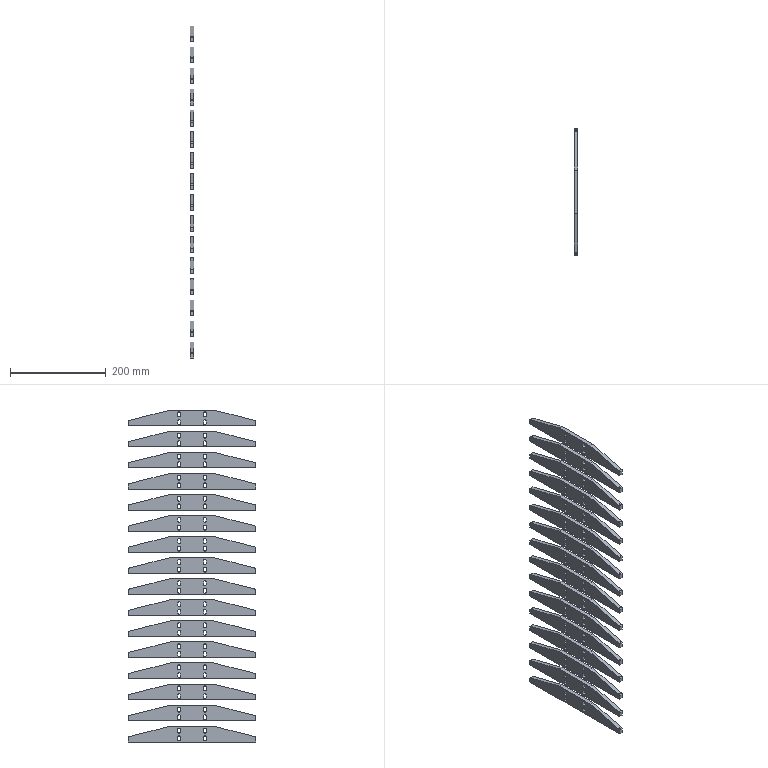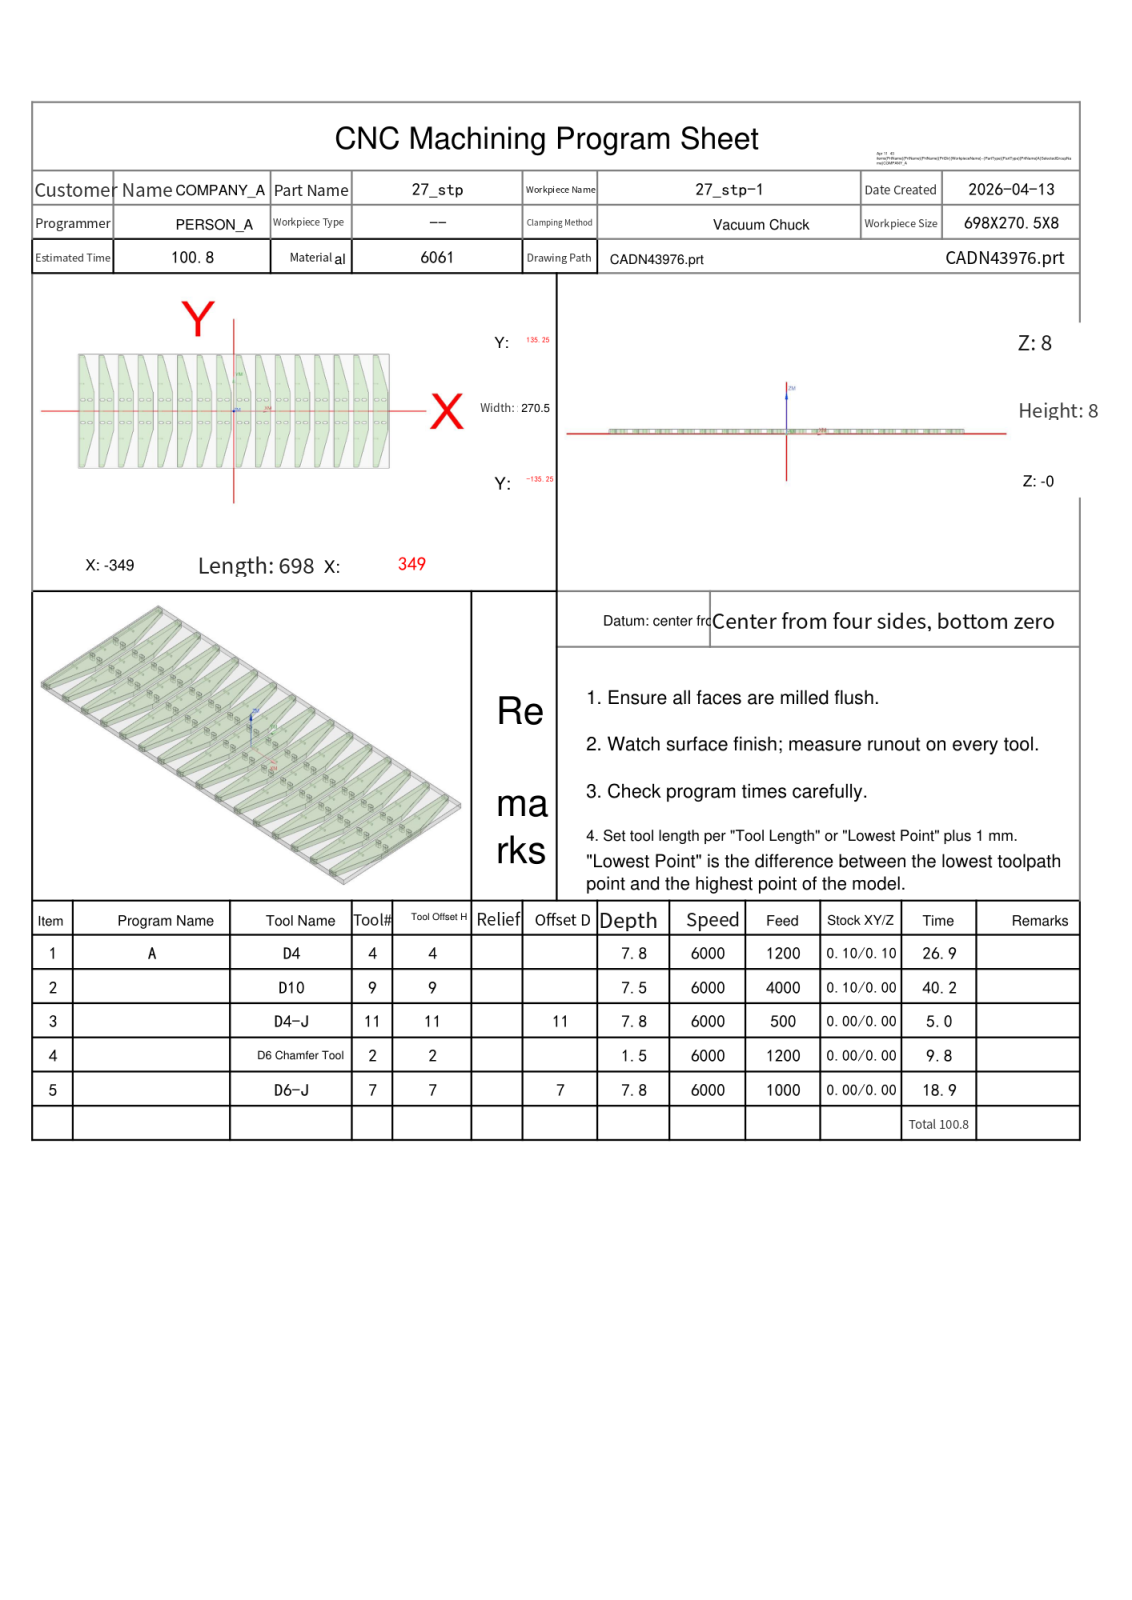NC program | NX | posted by the shop | part box 8 x 265.5 x 693 mm
Lines 17059 to 19371 of 21683, first 2178 of 2313 lines:
N3 T11 M06
(D4-J  D=4. R=0. H=11 ce=0.00 di=0.00)
G00 G90 G54 X-323. Y-27.5 M03 S6000
G43 H11 Z28.
M08
Z4.6
G01 Z4.1 F500.
G41 D11
Y-27.55
G03 X-322.8 Y-27.75 I.2 J0.0
G01 X-320.3
G03 X-319.55 Y-27. I0.0 J.75
X-320.3 Y-26.25 I-.75 J0.0
G01 X-325.3
G03 X-326.05 Y-27. I0.0 J-.75
X-325.3 Y-27.75 I.75 J0.0
G01 X-322.8
X-322.3
G03 X-322.1 Y-27.55 I0.0 J.2
G01 G40 Y-27.5
Z4.6
G00 Z9.
X-323.
Z.7
G01 Z.2
G41 D11
Y-27.55
G03 X-322.8 Y-27.75 I.2 J0.0
G01 X-320.3
G03 X-319.55 Y-27. I0.0 J.75
X-320.3 Y-26.25 I-.75 J0.0
G01 X-325.3
G03 X-326.05 Y-27. I0.0 J-.75
X-325.3 Y-27.75 I.75 J0.0
G01 X-322.8
X-322.3
G03 X-322.1 Y-27.55 I0.0 J.2
G01 G40 Y-27.5
Z.7
G00 Z28.
X-338.6 Y-26.5
Z4.6
G01 Z4.1
G41 D11
Y-26.45
G03 X-338.8 Y-26.25 I-.2 J0.0
G01 X-341.3
G03 X-342.05 Y-27. I0.0 J-.75
X-341.3 Y-27.75 I.75 J0.0
G01 X-336.3
G03 X-335.55 Y-27. I0.0 J.75
X-336.3 Y-26.25 I-.75 J0.0
G01 X-338.8
X-339.3
G03 X-339.5 Y-26.45 I0.0 J-.2
G01 G40 Y-26.5
Z4.6
G00 Z9.
X-338.6
Z.7
G01 Z.2
G41 D11
Y-26.45
G03 X-338.8 Y-26.25 I-.2 J0.0
G01 X-341.3
G03 X-342.05 Y-27. I0.0 J-.75
X-341.3 Y-27.75 I.75 J0.0
G01 X-336.3
G03 X-335.55 Y-27. I0.0 J.75
X-336.3 Y-26.25 I-.75 J0.0
G01 X-338.8
X-339.3
G03 X-339.5 Y-26.45 I0.0 J-.2
G01 G40 Y-26.5
Z.7
G00 Z28.
X-278.6
Z4.6
G01 Z4.1
G41 D11
Y-26.45
G03 X-278.8 Y-26.25 I-.2 J0.0
G01 X-281.3
G03 X-282.05 Y-27. I0.0 J-.75
X-281.3 Y-27.75 I.75 J0.0
G01 X-276.3
G03 X-275.55 Y-27. I0.0 J.75
X-276.3 Y-26.25 I-.75 J0.0
G01 X-278.8
X-279.3
G03 X-279.5 Y-26.45 I0.0 J-.2
G01 G40 Y-26.5
Z4.6
G00 Z9.
X-278.6
Z.7
G01 Z.2
G41 D11
Y-26.45
G03 X-278.8 Y-26.25 I-.2 J0.0
G01 X-281.3
G03 X-282.05 Y-27. I0.0 J-.75
X-281.3 Y-27.75 I.75 J0.0
G01 X-276.3
G03 X-275.55 Y-27. I0.0 J.75
X-276.3 Y-26.25 I-.75 J0.0
G01 X-278.8
X-279.3
G03 X-279.5 Y-26.45 I0.0 J-.2
G01 G40 Y-26.5
Z.7
G00 Z28.
X-294.6
Z4.6
G01 Z4.1
G41 D11
Y-26.45
G03 X-294.8 Y-26.25 I-.2 J0.0
G01 X-297.3
G03 X-298.05 Y-27. I0.0 J-.75
X-297.3 Y-27.75 I.75 J0.0
G01 X-292.3
G03 X-291.55 Y-27. I0.0 J.75
X-292.3 Y-26.25 I-.75 J0.0
G01 X-294.8
X-295.3
G03 X-295.5 Y-26.45 I0.0 J-.2
G01 G40 Y-26.5
Z4.6
G00 Z9.
X-294.6
Z.7
G01 Z.2
G41 D11
Y-26.45
G03 X-294.8 Y-26.25 I-.2 J0.0
G01 X-297.3
G03 X-298.05 Y-27. I0.0 J-.75
X-297.3 Y-27.75 I.75 J0.0
G01 X-292.3
G03 X-291.55 Y-27. I0.0 J.75
X-292.3 Y-26.25 I-.75 J0.0
G01 X-294.8
X-295.3
G03 X-295.5 Y-26.45 I0.0 J-.2
G01 G40 Y-26.5
Z.7
G00 Z28.
X-235. Y-27.5
Z4.6
G01 Z4.1
G41 D11
Y-27.55
G03 X-234.8 Y-27.75 I.2 J0.0
G01 X-232.3
G03 X-231.55 Y-27. I0.0 J.75
X-232.3 Y-26.25 I-.75 J0.0
G01 X-237.3
G03 X-238.05 Y-27. I0.0 J-.75
X-237.3 Y-27.75 I.75 J0.0
G01 X-234.8
X-234.3
G03 X-234.1 Y-27.55 I0.0 J.2
G01 G40 Y-27.5
Z4.6
G00 Z9.
X-235.
Z.7
G01 Z.2
G41 D11
Y-27.55
G03 X-234.8 Y-27.75 I.2 J0.0
G01 X-232.3
G03 X-231.55 Y-27. I0.0 J.75
X-232.3 Y-26.25 I-.75 J0.0
G01 X-237.3
G03 X-238.05 Y-27. I0.0 J-.75
X-237.3 Y-27.75 I.75 J0.0
G01 X-234.8
X-234.3
G03 X-234.1 Y-27.55 I0.0 J.2
G01 G40 Y-27.5
Z.7
G00 Z28.
X-251.
Z4.6
G01 Z4.1
G41 D11
Y-27.55
G03 X-250.8 Y-27.75 I.2 J0.0
G01 X-248.3
G03 X-247.55 Y-27. I0.0 J.75
X-248.3 Y-26.25 I-.75 J0.0
G01 X-253.3
G03 X-254.05 Y-27. I0.0 J-.75
X-253.3 Y-27.75 I.75 J0.0
G01 X-250.8
X-250.3
G03 X-250.1 Y-27.55 I0.0 J.2
G01 G40 Y-27.5
Z4.6
G00 Z9.
X-251.
Z.7
G01 Z.2
G41 D11
Y-27.55
G03 X-250.8 Y-27.75 I.2 J0.0
G01 X-248.3
G03 X-247.55 Y-27. I0.0 J.75
X-248.3 Y-26.25 I-.75 J0.0
G01 X-253.3
G03 X-254.05 Y-27. I0.0 J-.75
X-253.3 Y-27.75 I.75 J0.0
G01 X-250.8
X-250.3
G03 X-250.1 Y-27.55 I0.0 J.2
G01 G40 Y-27.5
Z.7
G00 Z28.
X-191.
Z4.6
G01 Z4.1
G41 D11
Y-27.55
G03 X-190.8 Y-27.75 I.2 J0.0
G01 X-188.3
G03 X-187.55 Y-27. I0.0 J.75
X-188.3 Y-26.25 I-.75 J0.0
G01 X-193.3
G03 X-194.05 Y-27. I0.0 J-.75
X-193.3 Y-27.75 I.75 J0.0
G01 X-190.8
X-190.3
G03 X-190.1 Y-27.55 I0.0 J.2
G01 G40 Y-27.5
Z4.6
G00 Z9.
X-191.
Z.7
G01 Z.2
G41 D11
Y-27.55
G03 X-190.8 Y-27.75 I.2 J0.0
G01 X-188.3
G03 X-187.55 Y-27. I0.0 J.75
X-188.3 Y-26.25 I-.75 J0.0
G01 X-193.3
G03 X-194.05 Y-27. I0.0 J-.75
X-193.3 Y-27.75 I.75 J0.0
G01 X-190.8
X-190.3
G03 X-190.1 Y-27.55 I0.0 J.2
G01 G40 Y-27.5
Z.7
G00 Z28.
X-207.
Z4.6
G01 Z4.1
G41 D11
Y-27.55
G03 X-206.8 Y-27.75 I.2 J0.0
G01 X-204.3
G03 X-203.55 Y-27. I0.0 J.75
X-204.3 Y-26.25 I-.75 J0.0
G01 X-209.3
G03 X-210.05 Y-27. I0.0 J-.75
X-209.3 Y-27.75 I.75 J0.0
G01 X-206.8
X-206.3
G03 X-206.1 Y-27.55 I0.0 J.2
G01 G40 Y-27.5
Z4.6
G00 Z9.
X-207.
Z.7
G01 Z.2
G41 D11
Y-27.55
G03 X-206.8 Y-27.75 I.2 J0.0
G01 X-204.3
G03 X-203.55 Y-27. I0.0 J.75
X-204.3 Y-26.25 I-.75 J0.0
G01 X-209.3
G03 X-210.05 Y-27. I0.0 J-.75
X-209.3 Y-27.75 I.75 J0.0
G01 X-206.8
X-206.3
G03 X-206.1 Y-27.55 I0.0 J.2
G01 G40 Y-27.5
Z.7
G00 Z28.
X-147.
Z4.6
G01 Z4.1
G41 D11
Y-27.55
G03 X-146.8 Y-27.75 I.2 J0.0
G01 X-144.3
G03 X-143.55 Y-27. I0.0 J.75
X-144.3 Y-26.25 I-.75 J0.0
G01 X-149.3
G03 X-150.05 Y-27. I0.0 J-.75
X-149.3 Y-27.75 I.75 J0.0
G01 X-146.8
X-146.3
G03 X-146.1 Y-27.55 I0.0 J.2
G01 G40 Y-27.5
Z4.6
G00 Z9.
X-147.
Z.7
G01 Z.2
G41 D11
Y-27.55
G03 X-146.8 Y-27.75 I.2 J0.0
G01 X-144.3
G03 X-143.55 Y-27. I0.0 J.75
X-144.3 Y-26.25 I-.75 J0.0
G01 X-149.3
G03 X-150.05 Y-27. I0.0 J-.75
X-149.3 Y-27.75 I.75 J0.0
G01 X-146.8
X-146.3
G03 X-146.1 Y-27.55 I0.0 J.2
G01 G40 Y-27.5
Z.7
G00 Z28.
X-163.
Z4.6
G01 Z4.1
G41 D11
Y-27.55
G03 X-162.8 Y-27.75 I.2 J0.0
G01 X-160.3
G03 X-159.55 Y-27. I0.0 J.75
X-160.3 Y-26.25 I-.75 J0.0
G01 X-165.3
G03 X-166.05 Y-27. I0.0 J-.75
X-165.3 Y-27.75 I.75 J0.0
G01 X-162.8
X-162.3
G03 X-162.1 Y-27.55 I0.0 J.2
G01 G40 Y-27.5
Z4.6
G00 Z9.
X-163.
Z.7
G01 Z.2
G41 D11
Y-27.55
G03 X-162.8 Y-27.75 I.2 J0.0
G01 X-160.3
G03 X-159.55 Y-27. I0.0 J.75
X-160.3 Y-26.25 I-.75 J0.0
G01 X-165.3
G03 X-166.05 Y-27. I0.0 J-.75
X-165.3 Y-27.75 I.75 J0.0
G01 X-162.8
X-162.3
G03 X-162.1 Y-27.55 I0.0 J.2
G01 G40 Y-27.5
Z.7
G00 Z28.
X-103.
Z4.6
G01 Z4.1
G41 D11
Y-27.55
G03 X-102.8 Y-27.75 I.2 J0.0
G01 X-100.3
G03 X-99.55 Y-27. I0.0 J.75
X-100.3 Y-26.25 I-.75 J0.0
G01 X-105.3
G03 X-106.05 Y-27. I0.0 J-.75
X-105.3 Y-27.75 I.75 J0.0
G01 X-102.8
X-102.3
G03 X-102.1 Y-27.55 I0.0 J.2
G01 G40 Y-27.5
Z4.6
G00 Z9.
X-103.
Z.7
G01 Z.2
G41 D11
Y-27.55
G03 X-102.8 Y-27.75 I.2 J0.0
G01 X-100.3
G03 X-99.55 Y-27. I0.0 J.75
X-100.3 Y-26.25 I-.75 J0.0
G01 X-105.3
G03 X-106.05 Y-27. I0.0 J-.75
X-105.3 Y-27.75 I.75 J0.0
G01 X-102.8
X-102.3
G03 X-102.1 Y-27.55 I0.0 J.2
G01 G40 Y-27.5
Z.7
G00 Z28.
X-119.
Z4.6
G01 Z4.1
G41 D11
Y-27.55
G03 X-118.8 Y-27.75 I.2 J0.0
G01 X-116.3
G03 X-115.55 Y-27. I0.0 J.75
X-116.3 Y-26.25 I-.75 J0.0
G01 X-121.3
G03 X-122.05 Y-27. I0.0 J-.75
X-121.3 Y-27.75 I.75 J0.0
G01 X-118.8
X-118.3
G03 X-118.1 Y-27.55 I0.0 J.2
G01 G40 Y-27.5
Z4.6
G00 Z9.
X-119.
Z.7
G01 Z.2
G41 D11
Y-27.55
G03 X-118.8 Y-27.75 I.2 J0.0
G01 X-116.3
G03 X-115.55 Y-27. I0.0 J.75
X-116.3 Y-26.25 I-.75 J0.0
G01 X-121.3
G03 X-122.05 Y-27. I0.0 J-.75
X-121.3 Y-27.75 I.75 J0.0
G01 X-118.8
X-118.3
G03 X-118.1 Y-27.55 I0.0 J.2
G01 G40 Y-27.5
Z.7
G00 Z28.
X-59.
Z4.6
G01 Z4.1
G41 D11
Y-27.55
G03 X-58.8 Y-27.75 I.2 J0.0
G01 X-56.3
G03 X-55.55 Y-27. I0.0 J.75
X-56.3 Y-26.25 I-.75 J0.0
G01 X-61.3
G03 X-62.05 Y-27. I0.0 J-.75
X-61.3 Y-27.75 I.75 J0.0
G01 X-58.8
X-58.3
G03 X-58.1 Y-27.55 I0.0 J.2
G01 G40 Y-27.5
Z4.6
G00 Z9.
X-59.
Z.7
G01 Z.2
G41 D11
Y-27.55
G03 X-58.8 Y-27.75 I.2 J0.0
G01 X-56.3
G03 X-55.55 Y-27. I0.0 J.75
X-56.3 Y-26.25 I-.75 J0.0
G01 X-61.3
G03 X-62.05 Y-27. I0.0 J-.75
X-61.3 Y-27.75 I.75 J0.0
G01 X-58.8
X-58.3
G03 X-58.1 Y-27.55 I0.0 J.2
G01 G40 Y-27.5
Z.7
G00 Z28.
X-75.
Z4.6
G01 Z4.1
G41 D11
Y-27.55
G03 X-74.8 Y-27.75 I.2 J0.0
G01 X-72.3
G03 X-71.55 Y-27. I0.0 J.75
X-72.3 Y-26.25 I-.75 J0.0
G01 X-77.3
G03 X-78.05 Y-27. I0.0 J-.75
X-77.3 Y-27.75 I.75 J0.0
G01 X-74.8
X-74.3
G03 X-74.1 Y-27.55 I0.0 J.2
G01 G40 Y-27.5
Z4.6
G00 Z9.
X-75.
Z.7
G01 Z.2
G41 D11
Y-27.55
G03 X-74.8 Y-27.75 I.2 J0.0
G01 X-72.3
G03 X-71.55 Y-27. I0.0 J.75
X-72.3 Y-26.25 I-.75 J0.0
G01 X-77.3
G03 X-78.05 Y-27. I0.0 J-.75
X-77.3 Y-27.75 I.75 J0.0
G01 X-74.8
X-74.3
G03 X-74.1 Y-27.55 I0.0 J.2
G01 G40 Y-27.5
Z.7
G00 Z28.
X-15.
Z4.6
G01 Z4.1
G41 D11
Y-27.55
G03 X-14.8 Y-27.75 I.2 J0.0
G01 X-12.3
G03 X-11.55 Y-27. I0.0 J.75
X-12.3 Y-26.25 I-.75 J0.0
G01 X-17.3
G03 X-18.05 Y-27. I0.0 J-.75
X-17.3 Y-27.75 I.75 J0.0
G01 X-14.8
X-14.3
G03 X-14.1 Y-27.55 I0.0 J.2
G01 G40 Y-27.5
Z4.6
G00 Z9.
X-15.
Z.7
G01 Z.2
G41 D11
Y-27.55
G03 X-14.8 Y-27.75 I.2 J0.0
G01 X-12.3
G03 X-11.55 Y-27. I0.0 J.75
X-12.3 Y-26.25 I-.75 J0.0
G01 X-17.3
G03 X-18.05 Y-27. I0.0 J-.75
X-17.3 Y-27.75 I.75 J0.0
G01 X-14.8
X-14.3
G03 X-14.1 Y-27.55 I0.0 J.2
G01 G40 Y-27.5
Z.7
G00 Z28.
X-31.
Z4.6
G01 Z4.1
G41 D11
Y-27.55
G03 X-30.8 Y-27.75 I.2 J0.0
G01 X-28.3
G03 X-27.55 Y-27. I0.0 J.75
X-28.3 Y-26.25 I-.75 J0.0
G01 X-33.3
G03 X-34.05 Y-27. I0.0 J-.75
X-33.3 Y-27.75 I.75 J0.0
G01 X-30.8
X-30.3
G03 X-30.1 Y-27.55 I0.0 J.2
G01 G40 Y-27.5
Z4.6
G00 Z9.
X-31.
Z.7
G01 Z.2
G41 D11
Y-27.55
G03 X-30.8 Y-27.75 I.2 J0.0
G01 X-28.3
G03 X-27.55 Y-27. I0.0 J.75
X-28.3 Y-26.25 I-.75 J0.0
G01 X-33.3
G03 X-34.05 Y-27. I0.0 J-.75
X-33.3 Y-27.75 I.75 J0.0
G01 X-30.8
X-30.3
G03 X-30.1 Y-27.55 I0.0 J.2
G01 G40 Y-27.5
Z.7
G00 Z28.
X29.
Z4.6
G01 Z4.1
G41 D11
Y-27.55
G03 X29.2 Y-27.75 I.2 J0.0
G01 X31.7
G03 X32.45 Y-27. I0.0 J.75
X31.7 Y-26.25 I-.75 J0.0
G01 X26.7
G03 X25.95 Y-27. I0.0 J-.75
X26.7 Y-27.75 I.75 J0.0
G01 X29.2
X29.7
G03 X29.9 Y-27.55 I0.0 J.2
G01 G40 Y-27.5
Z4.6
G00 Z9.
X29.
Z.7
G01 Z.2
G41 D11
Y-27.55
G03 X29.2 Y-27.75 I.2 J0.0
G01 X31.7
G03 X32.45 Y-27. I0.0 J.75
X31.7 Y-26.25 I-.75 J0.0
G01 X26.7
G03 X25.95 Y-27. I0.0 J-.75
X26.7 Y-27.75 I.75 J0.0
G01 X29.2
X29.7
G03 X29.9 Y-27.55 I0.0 J.2
G01 G40 Y-27.5
Z.7
G00 Z28.
X13.
Z4.6
G01 Z4.1
G41 D11
Y-27.55
G03 X13.2 Y-27.75 I.2 J0.0
G01 X15.7
G03 X16.45 Y-27. I0.0 J.75
X15.7 Y-26.25 I-.75 J0.0
G01 X10.7
G03 X9.95 Y-27. I0.0 J-.75
X10.7 Y-27.75 I.75 J0.0
G01 X13.2
X13.7
G03 X13.9 Y-27.55 I0.0 J.2
G01 G40 Y-27.5
Z4.6
G00 Z9.
X13.
Z.7
G01 Z.2
G41 D11
Y-27.55
G03 X13.2 Y-27.75 I.2 J0.0
G01 X15.7
G03 X16.45 Y-27. I0.0 J.75
X15.7 Y-26.25 I-.75 J0.0
G01 X10.7
G03 X9.95 Y-27. I0.0 J-.75
X10.7 Y-27.75 I.75 J0.0
G01 X13.2
X13.7
G03 X13.9 Y-27.55 I0.0 J.2
G01 G40 Y-27.5
Z.7
G00 Z28.
X73.
Z4.6
G01 Z4.1
G41 D11
Y-27.55
G03 X73.2 Y-27.75 I.2 J0.0
G01 X75.7
G03 X76.45 Y-27. I0.0 J.75
X75.7 Y-26.25 I-.75 J0.0
G01 X70.7
G03 X69.95 Y-27. I0.0 J-.75
X70.7 Y-27.75 I.75 J0.0
G01 X73.2
X73.7
G03 X73.9 Y-27.55 I0.0 J.2
G01 G40 Y-27.5
Z4.6
G00 Z9.
X73.
Z.7
G01 Z.2
G41 D11
Y-27.55
G03 X73.2 Y-27.75 I.2 J0.0
G01 X75.7
G03 X76.45 Y-27. I0.0 J.75
X75.7 Y-26.25 I-.75 J0.0
G01 X70.7
G03 X69.95 Y-27. I0.0 J-.75
X70.7 Y-27.75 I.75 J0.0
G01 X73.2
X73.7
G03 X73.9 Y-27.55 I0.0 J.2
G01 G40 Y-27.5
Z.7
G00 Z28.
X57.
Z4.6
G01 Z4.1
G41 D11
Y-27.55
G03 X57.2 Y-27.75 I.2 J0.0
G01 X59.7
G03 X60.45 Y-27. I0.0 J.75
X59.7 Y-26.25 I-.75 J0.0
G01 X54.7
G03 X53.95 Y-27. I0.0 J-.75
X54.7 Y-27.75 I.75 J0.0
G01 X57.2
X57.7
G03 X57.9 Y-27.55 I0.0 J.2
G01 G40 Y-27.5
Z4.6
G00 Z9.
X57.
Z.7
G01 Z.2
G41 D11
Y-27.55
G03 X57.2 Y-27.75 I.2 J0.0
G01 X59.7
G03 X60.45 Y-27. I0.0 J.75
X59.7 Y-26.25 I-.75 J0.0
G01 X54.7
G03 X53.95 Y-27. I0.0 J-.75
X54.7 Y-27.75 I.75 J0.0
G01 X57.2
X57.7
G03 X57.9 Y-27.55 I0.0 J.2
G01 G40 Y-27.5
Z.7
G00 Z28.
X117.
Z4.6
G01 Z4.1
G41 D11
Y-27.55
G03 X117.2 Y-27.75 I.2 J0.0
G01 X119.7
G03 X120.45 Y-27. I0.0 J.75
X119.7 Y-26.25 I-.75 J0.0
G01 X114.7
G03 X113.95 Y-27. I0.0 J-.75
X114.7 Y-27.75 I.75 J0.0
G01 X117.2
X117.7
G03 X117.9 Y-27.55 I0.0 J.2
G01 G40 Y-27.5
Z4.6
G00 Z9.
X117.
Z.7
G01 Z.2
G41 D11
Y-27.55
G03 X117.2 Y-27.75 I.2 J0.0
G01 X119.7
G03 X120.45 Y-27. I0.0 J.75
X119.7 Y-26.25 I-.75 J0.0
G01 X114.7
G03 X113.95 Y-27. I0.0 J-.75
X114.7 Y-27.75 I.75 J0.0
G01 X117.2
X117.7
G03 X117.9 Y-27.55 I0.0 J.2
G01 G40 Y-27.5
Z.7
G00 Z28.
X101.
Z4.6
G01 Z4.1
G41 D11
Y-27.55
G03 X101.2 Y-27.75 I.2 J0.0
G01 X103.7
G03 X104.45 Y-27. I0.0 J.75
X103.7 Y-26.25 I-.75 J0.0
G01 X98.7
G03 X97.95 Y-27. I0.0 J-.75
X98.7 Y-27.75 I.75 J0.0
G01 X101.2
X101.7
G03 X101.9 Y-27.55 I0.0 J.2
G01 G40 Y-27.5
Z4.6
G00 Z9.
X101.
Z.7
G01 Z.2
G41 D11
Y-27.55
G03 X101.2 Y-27.75 I.2 J0.0
G01 X103.7
G03 X104.45 Y-27. I0.0 J.75
X103.7 Y-26.25 I-.75 J0.0
G01 X98.7
G03 X97.95 Y-27. I0.0 J-.75
X98.7 Y-27.75 I.75 J0.0
G01 X101.2
X101.7
G03 X101.9 Y-27.55 I0.0 J.2
G01 G40 Y-27.5
Z.7
G00 Z28.
X161.
Z4.6
G01 Z4.1
G41 D11
Y-27.55
G03 X161.2 Y-27.75 I.2 J0.0
G01 X163.7
G03 X164.45 Y-27. I0.0 J.75
X163.7 Y-26.25 I-.75 J0.0
G01 X158.7
G03 X157.95 Y-27. I0.0 J-.75
X158.7 Y-27.75 I.75 J0.0
G01 X161.2
X161.7
G03 X161.9 Y-27.55 I0.0 J.2
G01 G40 Y-27.5
Z4.6
G00 Z9.
X161.
Z.7
G01 Z.2
G41 D11
Y-27.55
G03 X161.2 Y-27.75 I.2 J0.0
G01 X163.7
G03 X164.45 Y-27. I0.0 J.75
X163.7 Y-26.25 I-.75 J0.0
G01 X158.7
G03 X157.95 Y-27. I0.0 J-.75
X158.7 Y-27.75 I.75 J0.0
G01 X161.2
X161.7
G03 X161.9 Y-27.55 I0.0 J.2
G01 G40 Y-27.5
Z.7
G00 Z28.
X145.
Z4.6
G01 Z4.1
G41 D11
Y-27.55
G03 X145.2 Y-27.75 I.2 J0.0
G01 X147.7
G03 X148.45 Y-27. I0.0 J.75
X147.7 Y-26.25 I-.75 J0.0
G01 X142.7
G03 X141.95 Y-27. I0.0 J-.75
X142.7 Y-27.75 I.75 J0.0
G01 X145.2
X145.7
G03 X145.9 Y-27.55 I0.0 J.2
G01 G40 Y-27.5
Z4.6
G00 Z9.
X145.
Z.7
G01 Z.2
G41 D11
Y-27.55
G03 X145.2 Y-27.75 I.2 J0.0
G01 X147.7
G03 X148.45 Y-27. I0.0 J.75
X147.7 Y-26.25 I-.75 J0.0
G01 X142.7
G03 X141.95 Y-27. I0.0 J-.75
X142.7 Y-27.75 I.75 J0.0
G01 X145.2
X145.7
G03 X145.9 Y-27.55 I0.0 J.2
G01 G40 Y-27.5
Z.7
G00 Z28.
X205.
Z4.6
G01 Z4.1
G41 D11
Y-27.55
G03 X205.2 Y-27.75 I.2 J0.0
G01 X207.7
G03 X208.45 Y-27. I0.0 J.75
X207.7 Y-26.25 I-.75 J0.0
G01 X202.7
G03 X201.95 Y-27. I0.0 J-.75
X202.7 Y-27.75 I.75 J0.0
G01 X205.2
X205.7
G03 X205.9 Y-27.55 I0.0 J.2
G01 G40 Y-27.5
Z4.6
G00 Z9.
X205.
Z.7
G01 Z.2
G41 D11
Y-27.55
G03 X205.2 Y-27.75 I.2 J0.0
G01 X207.7
G03 X208.45 Y-27. I0.0 J.75
X207.7 Y-26.25 I-.75 J0.0
G01 X202.7
G03 X201.95 Y-27. I0.0 J-.75
X202.7 Y-27.75 I.75 J0.0
G01 X205.2
X205.7
G03 X205.9 Y-27.55 I0.0 J.2
G01 G40 Y-27.5
Z.7
G00 Z28.
X189.
Z4.6
G01 Z4.1
G41 D11
Y-27.55
G03 X189.2 Y-27.75 I.2 J0.0
G01 X191.7
G03 X192.45 Y-27. I0.0 J.75
X191.7 Y-26.25 I-.75 J0.0
G01 X186.7
G03 X185.95 Y-27. I0.0 J-.75
X186.7 Y-27.75 I.75 J0.0
G01 X189.2
X189.7
G03 X189.9 Y-27.55 I0.0 J.2
G01 G40 Y-27.5
Z4.6
G00 Z9.
X189.
Z.7
G01 Z.2
G41 D11
Y-27.55
G03 X189.2 Y-27.75 I.2 J0.0
G01 X191.7
G03 X192.45 Y-27. I0.0 J.75
X191.7 Y-26.25 I-.75 J0.0
G01 X186.7
G03 X185.95 Y-27. I0.0 J-.75
X186.7 Y-27.75 I.75 J0.0
G01 X189.2
X189.7
G03 X189.9 Y-27.55 I0.0 J.2
G01 G40 Y-27.5
Z.7
G00 Z28.
X249.
Z4.6
G01 Z4.1
G41 D11
Y-27.55
G03 X249.2 Y-27.75 I.2 J0.0
G01 X251.7
G03 X252.45 Y-27. I0.0 J.75
X251.7 Y-26.25 I-.75 J0.0
G01 X246.7
G03 X245.95 Y-27. I0.0 J-.75
X246.7 Y-27.75 I.75 J0.0
G01 X249.2
X249.7
G03 X249.9 Y-27.55 I0.0 J.2
G01 G40 Y-27.5
Z4.6
G00 Z9.
X249.
Z.7
G01 Z.2
G41 D11
Y-27.55
G03 X249.2 Y-27.75 I.2 J0.0
G01 X251.7
G03 X252.45 Y-27. I0.0 J.75
X251.7 Y-26.25 I-.75 J0.0
G01 X246.7
G03 X245.95 Y-27. I0.0 J-.75
X246.7 Y-27.75 I.75 J0.0
G01 X249.2
X249.7
G03 X249.9 Y-27.55 I0.0 J.2
G01 G40 Y-27.5
Z.7
G00 Z28.
X233.
Z4.6
G01 Z4.1
G41 D11
Y-27.55
G03 X233.2 Y-27.75 I.2 J0.0
G01 X235.7
G03 X236.45 Y-27. I0.0 J.75
X235.7 Y-26.25 I-.75 J0.0
G01 X230.7
G03 X229.95 Y-27. I0.0 J-.75
X230.7 Y-27.75 I.75 J0.0
G01 X233.2
X233.7
G03 X233.9 Y-27.55 I0.0 J.2
G01 G40 Y-27.5
Z4.6
G00 Z9.
X233.
Z.7
G01 Z.2
G41 D11
Y-27.55
G03 X233.2 Y-27.75 I.2 J0.0
G01 X235.7
G03 X236.45 Y-27. I0.0 J.75
X235.7 Y-26.25 I-.75 J0.0
G01 X230.7
G03 X229.95 Y-27. I0.0 J-.75
X230.7 Y-27.75 I.75 J0.0
G01 X233.2
X233.7
G03 X233.9 Y-27.55 I0.0 J.2
G01 G40 Y-27.5
Z.7
G00 Z28.
X293.
Z4.6
G01 Z4.1
G41 D11
Y-27.55
G03 X293.2 Y-27.75 I.2 J0.0
G01 X295.7
G03 X296.45 Y-27. I0.0 J.75
X295.7 Y-26.25 I-.75 J0.0
G01 X290.7
G03 X289.95 Y-27. I0.0 J-.75
X290.7 Y-27.75 I.75 J0.0
G01 X293.2
X293.7
G03 X293.9 Y-27.55 I0.0 J.2
G01 G40 Y-27.5
Z4.6
G00 Z9.
X293.
Z.7
G01 Z.2
G41 D11
Y-27.55
G03 X293.2 Y-27.75 I.2 J0.0
G01 X295.7
G03 X296.45 Y-27. I0.0 J.75
X295.7 Y-26.25 I-.75 J0.0
G01 X290.7
G03 X289.95 Y-27. I0.0 J-.75
X290.7 Y-27.75 I.75 J0.0
G01 X293.2
X293.7
G03 X293.9 Y-27.55 I0.0 J.2
G01 G40 Y-27.5
Z.7
G00 Z28.
X277.4 Y-26.5
Z4.6
G01 Z4.1
G41 D11
Y-26.45
G03 X277.2 Y-26.25 I-.2 J0.0
G01 X274.7
G03 X273.95 Y-27. I0.0 J-.75
X274.7 Y-27.75 I.75 J0.0
G01 X279.7
G03 X280.45 Y-27. I0.0 J.75
X279.7 Y-26.25 I-.75 J0.0
G01 X277.2
X276.7
G03 X276.5 Y-26.45 I0.0 J-.2
G01 G40 Y-26.5
Z4.6
G00 Z9.
X277.4
Z.7
G01 Z.2
G41 D11
Y-26.45
G03 X277.2 Y-26.25 I-.2 J0.0
G01 X274.7
G03 X273.95 Y-27. I0.0 J-.75
X274.7 Y-27.75 I.75 J0.0
G01 X279.7
G03 X280.45 Y-27. I0.0 J.75
X279.7 Y-26.25 I-.75 J0.0
G01 X277.2
X276.7
G03 X276.5 Y-26.45 I0.0 J-.2
G01 G40 Y-26.5
Z.7
G00 Z28.
X337.023 Y-27.5
Z4.6
G01 Z4.1
G41 D11
Y-27.55
G03 X337.223 Y-27.75 I.2 J0.0
G01 X339.7
G03 X340.45 Y-27. I0.0 J.75
X339.7 Y-26.25 I-.75 J0.0
G01 X334.7
G03 X333.95 Y-27. I0.0 J-.75
X334.7 Y-27.75 I.75 J0.0
G01 X337.223
X337.723
G03 X337.923 Y-27.55 I0.0 J.2
G01 G40 Y-27.5
Z4.6
G00 Z9.
X337.023
Z.7
G01 Z.2
G41 D11
Y-27.55
G03 X337.223 Y-27.75 I.2 J0.0
G01 X339.7
G03 X340.45 Y-27. I0.0 J.75
X339.7 Y-26.25 I-.75 J0.0
G01 X334.7
G03 X333.95 Y-27. I0.0 J-.75
X334.7 Y-27.75 I.75 J0.0
G01 X337.223
X337.723
G03 X337.923 Y-27.55 I0.0 J.2
G01 G40 Y-27.5
Z.7
G00 Z28.
X321.4 Y-26.5
Z4.6
G01 Z4.1
G41 D11
Y-26.45
G03 X321.2 Y-26.25 I-.2 J0.0
G01 X318.7
G03 X317.95 Y-27. I0.0 J-.75
X318.7 Y-27.75 I.75 J0.0
G01 X323.7
G03 X324.45 Y-27. I0.0 J.75
X323.7 Y-26.25 I-.75 J0.0
G01 X321.2
X320.7
G03 X320.5 Y-26.45 I0.0 J-.2
G01 G40 Y-26.5
Z4.6
G00 Z9.
X321.4
Z.7
G01 Z.2
G41 D11
Y-26.45
G03 X321.2 Y-26.25 I-.2 J0.0
G01 X318.7
G03 X317.95 Y-27. I0.0 J-.75
X318.7 Y-27.75 I.75 J0.0
G01 X323.7
G03 X324.45 Y-27. I0.0 J.75
X323.7 Y-26.25 I-.75 J0.0
G01 X321.2
X320.7
G03 X320.5 Y-26.45 I0.0 J-.2
G01 G40 Y-26.5
Z.7
G00 Z28.
X321. Y26.5
Z4.6
G01 Z4.1
G41 D11
Y26.45
G03 X321.2 Y26.25 I.2 J0.0
G01 X323.7
G03 X324.45 Y27. I0.0 J.75
X323.7 Y27.75 I-.75 J0.0
G01 X318.7
G03 X317.95 Y27. I0.0 J-.75
X318.7 Y26.25 I.75 J0.0
G01 X321.2
X321.7
G03 X321.9 Y26.45 I0.0 J.2
G01 G40 Y26.5
Z4.6
G00 Z9.
X321.
Z.7
G01 Z.2
G41 D11
Y26.45
G03 X321.2 Y26.25 I.2 J0.0
G01 X323.7
G03 X324.45 Y27. I0.0 J.75
X323.7 Y27.75 I-.75 J0.0
G01 X318.7
G03 X317.95 Y27. I0.0 J-.75
X318.7 Y26.25 I.75 J0.0
G01 X321.2
X321.7
G03 X321.9 Y26.45 I0.0 J.2
G01 G40 Y26.5
Z.7
G00 Z28.
X337.4 Y27.5
Z4.6
G01 Z4.1
G41 D11
Y27.55
G03 X337.2 Y27.75 I-.2 J0.0
G01 X334.7
G03 X333.95 Y27. I0.0 J-.75
X334.7 Y26.25 I.75 J0.0
G01 X339.7
G03 X340.45 Y27. I0.0 J.75
X339.7 Y27.75 I-.75 J0.0
G01 X337.2
X336.7
G03 X336.5 Y27.55 I0.0 J-.2
G01 G40 Y27.5
Z4.6
G00 Z9.
X337.4
Z.7
G01 Z.2
G41 D11
Y27.55
G03 X337.2 Y27.75 I-.2 J0.0
G01 X334.7
G03 X333.95 Y27. I0.0 J-.75
X334.7 Y26.25 I.75 J0.0
G01 X339.7
G03 X340.45 Y27. I0.0 J.75
X339.7 Y27.75 I-.75 J0.0
G01 X337.2
X336.7
G03 X336.5 Y27.55 I0.0 J-.2
G01 G40 Y27.5
Z.7
G00 Z28.
X277. Y26.5
Z4.6
G01 Z4.1
G41 D11
Y26.45
G03 X277.2 Y26.25 I.2 J0.0
G01 X279.7
G03 X280.45 Y27. I0.0 J.75
X279.7 Y27.75 I-.75 J0.0
G01 X274.7
G03 X273.95 Y27. I0.0 J-.75
X274.7 Y26.25 I.75 J0.0
G01 X277.2
X277.7
G03 X277.9 Y26.45 I0.0 J.2
G01 G40 Y26.5
Z4.6
G00 Z9.
X277.
Z.7
G01 Z.2
G41 D11
Y26.45
G03 X277.2 Y26.25 I.2 J0.0
G01 X279.7
G03 X280.45 Y27. I0.0 J.75
X279.7 Y27.75 I-.75 J0.0
G01 X274.7
G03 X273.95 Y27. I0.0 J-.75
X274.7 Y26.25 I.75 J0.0
G01 X277.2
X277.7
G03 X277.9 Y26.45 I0.0 J.2
G01 G40 Y26.5
Z.7
G00 Z28.
X293.4 Y27.5
Z4.6
G01 Z4.1
G41 D11
Y27.55
G03 X293.2 Y27.75 I-.2 J0.0
G01 X290.7
G03 X289.95 Y27. I0.0 J-.75
X290.7 Y26.25 I.75 J0.0
G01 X295.7
G03 X296.45 Y27. I0.0 J.75
X295.7 Y27.75 I-.75 J0.0
G01 X293.2
X292.7
G03 X292.5 Y27.55 I0.0 J-.2
G01 G40 Y27.5
Z4.6
G00 Z9.
X293.4
Z.7
G01 Z.2
G41 D11
Y27.55
G03 X293.2 Y27.75 I-.2 J0.0
G01 X290.7
G03 X289.95 Y27. I0.0 J-.75
X290.7 Y26.25 I.75 J0.0
G01 X295.7
G03 X296.45 Y27. I0.0 J.75
X295.7 Y27.75 I-.75 J0.0
G01 X293.2
X292.7
G03 X292.5 Y27.55 I0.0 J-.2
G01 G40 Y27.5
Z.7
G00 Z28.
X233.4
Z4.6
G01 Z4.1
G41 D11
Y27.55
G03 X233.2 Y27.75 I-.2 J0.0
G01 X230.7
G03 X229.95 Y27. I0.0 J-.75
X230.7 Y26.25 I.75 J0.0
G01 X235.7
G03 X236.45 Y27. I0.0 J.75
X235.7 Y27.75 I-.75 J0.0
G01 X233.2
X232.7
G03 X232.5 Y27.55 I0.0 J-.2
G01 G40 Y27.5
Z4.6
G00 Z9.
X233.4
Z.7
G01 Z.2
G41 D11
Y27.55
G03 X233.2 Y27.75 I-.2 J0.0
G01 X230.7
G03 X229.95 Y27. I0.0 J-.75
X230.7 Y26.25 I.75 J0.0
G01 X235.7
G03 X236.45 Y27. I0.0 J.75
X235.7 Y27.75 I-.75 J0.0
G01 X233.2
X232.7
G03 X232.5 Y27.55 I0.0 J-.2
G01 G40 Y27.5
Z.7
G00 Z28.
X249. Y26.5
Z4.6
G01 Z4.1
G41 D11
Y26.45
G03 X249.2 Y26.25 I.2 J0.0
G01 X251.7
G03 X252.45 Y27. I0.0 J.75
X251.7 Y27.75 I-.75 J0.0
G01 X246.7
G03 X245.95 Y27. I0.0 J-.75
X246.7 Y26.25 I.75 J0.0
G01 X249.2
X249.7
G03 X249.9 Y26.45 I0.0 J.2
G01 G40 Y26.5
Z4.6
G00 Z9.
X249.
Z.7
G01 Z.2
G41 D11
Y26.45
G03 X249.2 Y26.25 I.2 J0.0
G01 X251.7
G03 X252.45 Y27. I0.0 J.75
X251.7 Y27.75 I-.75 J0.0
G01 X246.7
G03 X245.95 Y27. I0.0 J-.75
X246.7 Y26.25 I.75 J0.0
G01 X249.2
X249.7
G03 X249.9 Y26.45 I0.0 J.2
G01 G40 Y26.5
Z.7
G00 Z28.
X189.4 Y27.5
Z4.6
G01 Z4.1
G41 D11
Y27.55
G03 X189.2 Y27.75 I-.2 J0.0
G01 X186.7
G03 X185.95 Y27. I0.0 J-.75
X186.7 Y26.25 I.75 J0.0
G01 X191.7
G03 X192.45 Y27. I0.0 J.75
X191.7 Y27.75 I-.75 J0.0
G01 X189.2
X188.7
G03 X188.5 Y27.55 I0.0 J-.2
G01 G40 Y27.5
Z4.6
G00 Z9.
X189.4
Z.7
G01 Z.2
G41 D11
Y27.55
G03 X189.2 Y27.75 I-.2 J0.0
G01 X186.7
G03 X185.95 Y27. I0.0 J-.75
X186.7 Y26.25 I.75 J0.0
G01 X191.7
G03 X192.45 Y27. I0.0 J.75
X191.7 Y27.75 I-.75 J0.0
G01 X189.2
X188.7
G03 X188.5 Y27.55 I0.0 J-.2
G01 G40 Y27.5
Z.7
G00 Z28.
X205.4
Z4.6
G01 Z4.1
G41 D11
Y27.55
G03 X205.2 Y27.75 I-.2 J0.0
G01 X202.7
G03 X201.95 Y27. I0.0 J-.75
X202.7 Y26.25 I.75 J0.0
G01 X207.7
G03 X208.45 Y27. I0.0 J.75
X207.7 Y27.75 I-.75 J0.0
G01 X205.2
X204.7
G03 X204.5 Y27.55 I0.0 J-.2
G01 G40 Y27.5
Z4.6
G00 Z9.
X205.4
Z.7
G01 Z.2
G41 D11
Y27.55
G03 X205.2 Y27.75 I-.2 J0.0
G01 X202.7
G03 X201.95 Y27. I0.0 J-.75
X202.7 Y26.25 I.75 J0.0
G01 X207.7
G03 X208.45 Y27. I0.0 J.75
X207.7 Y27.75 I-.75 J0.0
G01 X205.2
X204.7
G03 X204.5 Y27.55 I0.0 J-.2
G01 G40 Y27.5
Z.7
G00 Z28.
X145.4
Z4.6
G01 Z4.1
G41 D11
Y27.55
G03 X145.2 Y27.75 I-.2 J0.0
G01 X142.7
G03 X141.95 Y27. I0.0 J-.75
X142.7 Y26.25 I.75 J0.0
G01 X147.7
G03 X148.45 Y27. I0.0 J.75
X147.7 Y27.75 I-.75 J0.0
G01 X145.2
X144.7
G03 X144.5 Y27.55 I0.0 J-.2
G01 G40 Y27.5
Z4.6
G00 Z9.
X145.4
Z.7
G01 Z.2
G41 D11
Y27.55
G03 X145.2 Y27.75 I-.2 J0.0
G01 X142.7
G03 X141.95 Y27. I0.0 J-.75
X142.7 Y26.25 I.75 J0.0
G01 X147.7
G03 X148.45 Y27. I0.0 J.75
X147.7 Y27.75 I-.75 J0.0
G01 X145.2
X144.7
G03 X144.5 Y27.55 I0.0 J-.2
G01 G40 Y27.5
Z.7
G00 Z28.
X161.4
Z4.6
G01 Z4.1
G41 D11
Y27.55
G03 X161.2 Y27.75 I-.2 J0.0
G01 X158.7
G03 X157.95 Y27. I0.0 J-.75
X158.7 Y26.25 I.75 J0.0
G01 X163.7
G03 X164.45 Y27. I0.0 J.75
X163.7 Y27.75 I-.75 J0.0
G01 X161.2
X160.7
G03 X160.5 Y27.55 I0.0 J-.2
G01 G40 Y27.5
Z4.6
G00 Z9.
X161.4
Z.7
G01 Z.2
G41 D11
Y27.55
G03 X161.2 Y27.75 I-.2 J0.0
G01 X158.7
G03 X157.95 Y27. I0.0 J-.75
X158.7 Y26.25 I.75 J0.0
G01 X163.7
G03 X164.45 Y27. I0.0 J.75
X163.7 Y27.75 I-.75 J0.0
G01 X161.2
X160.7
G03 X160.5 Y27.55 I0.0 J-.2
G01 G40 Y27.5
Z.7
G00 Z28.
X101.4
Z4.6
G01 Z4.1
G41 D11
Y27.55
G03 X101.2 Y27.75 I-.2 J0.0
G01 X98.7
G03 X97.95 Y27. I0.0 J-.75
X98.7 Y26.25 I.75 J0.0
G01 X103.7
G03 X104.45 Y27. I0.0 J.75
X103.7 Y27.75 I-.75 J0.0
G01 X101.2
X100.7
G03 X100.5 Y27.55 I0.0 J-.2
G01 G40 Y27.5
Z4.6
G00 Z9.
X101.4
Z.7
G01 Z.2
G41 D11
Y27.55
G03 X101.2 Y27.75 I-.2 J0.0
G01 X98.7
G03 X97.95 Y27. I0.0 J-.75
X98.7 Y26.25 I.75 J0.0
G01 X103.7
G03 X104.45 Y27. I0.0 J.75
X103.7 Y27.75 I-.75 J0.0
G01 X101.2
X100.7
G03 X100.5 Y27.55 I0.0 J-.2
G01 G40 Y27.5
Z.7
G00 Z28.
X117.4
Z4.6
G01 Z4.1
G41 D11
Y27.55
G03 X117.2 Y27.75 I-.2 J0.0
G01 X114.7
G03 X113.95 Y27. I0.0 J-.75
X114.7 Y26.25 I.75 J0.0
G01 X119.7
G03 X120.45 Y27. I0.0 J.75
X119.7 Y27.75 I-.75 J0.0
G01 X117.2
X116.7
G03 X116.5 Y27.55 I0.0 J-.2
G01 G40 Y27.5
Z4.6
G00 Z9.
X117.4
Z.7
G01 Z.2
G41 D11
Y27.55
G03 X117.2 Y27.75 I-.2 J0.0
G01 X114.7
G03 X113.95 Y27. I0.0 J-.75
X114.7 Y26.25 I.75 J0.0
G01 X119.7
G03 X120.45 Y27. I0.0 J.75
X119.7 Y27.75 I-.75 J0.0
G01 X117.2
X116.7
G03 X116.5 Y27.55 I0.0 J-.2
G01 G40 Y27.5
Z.7
G00 Z28.
X57.4
Z4.6
G01 Z4.1
G41 D11
Y27.55
G03 X57.2 Y27.75 I-.2 J0.0
G01 X54.7
G03 X53.95 Y27. I0.0 J-.75
X54.7 Y26.25 I.75 J0.0
G01 X59.7
G03 X60.45 Y27. I0.0 J.75
X59.7 Y27.75 I-.75 J0.0
G01 X57.2
X56.7
G03 X56.5 Y27.55 I0.0 J-.2
G01 G40 Y27.5
Z4.6
G00 Z9.
X57.4
Z.7
G01 Z.2
G41 D11
Y27.55
G03 X57.2 Y27.75 I-.2 J0.0
G01 X54.7
G03 X53.95 Y27. I0.0 J-.75
X54.7 Y26.25 I.75 J0.0
G01 X59.7
G03 X60.45 Y27. I0.0 J.75
X59.7 Y27.75 I-.75 J0.0
G01 X57.2
X56.7
G03 X56.5 Y27.55 I0.0 J-.2
G01 G40 Y27.5
Z.7
G00 Z28.
X73.4
Z4.6
G01 Z4.1
G41 D11
Y27.55
G03 X73.2 Y27.75 I-.2 J0.0
G01 X70.7
G03 X69.95 Y27. I0.0 J-.75
X70.7 Y26.25 I.75 J0.0
G01 X75.7
G03 X76.45 Y27. I0.0 J.75
X75.7 Y27.75 I-.75 J0.0
G01 X73.2
X72.7
G03 X72.5 Y27.55 I0.0 J-.2
G01 G40 Y27.5
Z4.6
G00 Z9.
X73.4
Z.7
G01 Z.2
G41 D11
Y27.55
G03 X73.2 Y27.75 I-.2 J0.0
G01 X70.7
G03 X69.95 Y27. I0.0 J-.75
X70.7 Y26.25 I.75 J0.0
G01 X75.7
G03 X76.45 Y27. I0.0 J.75
X75.7 Y27.75 I-.75 J0.0
G01 X73.2
X72.7
G03 X72.5 Y27.55 I0.0 J-.2
G01 G40 Y27.5
Z.7
G00 Z28.
X13.4
Z4.6
G01 Z4.1
G41 D11
Y27.55
G03 X13.2 Y27.75 I-.2 J0.0
G01 X10.7
G03 X9.95 Y27. I0.0 J-.75
X10.7 Y26.25 I.75 J0.0
G01 X15.7
G03 X16.45 Y27. I0.0 J.75
X15.7 Y27.75 I-.75 J0.0
G01 X13.2
X12.7
G03 X12.5 Y27.55 I0.0 J-.2
G01 G40 Y27.5
Z4.6
G00 Z9.
X13.4
Z.7
G01 Z.2
G41 D11
Y27.55
G03 X13.2 Y27.75 I-.2 J0.0
G01 X10.7
G03 X9.95 Y27. I0.0 J-.75
X10.7 Y26.25 I.75 J0.0
G01 X15.7
G03 X16.45 Y27. I0.0 J.75
X15.7 Y27.75 I-.75 J0.0
G01 X13.2
X12.7
G03 X12.5 Y27.55 I0.0 J-.2
G01 G40 Y27.5
Z.7
G00 Z28.
X29.4
Z4.6
G01 Z4.1
G41 D11
Y27.55
G03 X29.2 Y27.75 I-.2 J0.0
G01 X26.7
G03 X25.95 Y27. I0.0 J-.75
X26.7 Y26.25 I.75 J0.0
G01 X31.7
G03 X32.45 Y27. I0.0 J.75
X31.7 Y27.75 I-.75 J0.0
G01 X29.2
X28.7
G03 X28.5 Y27.55 I0.0 J-.2
G01 G40 Y27.5
Z4.6
G00 Z9.
X29.4
Z.7
G01 Z.2
G41 D11
Y27.55
G03 X29.2 Y27.75 I-.2 J0.0
G01 X26.7
G03 X25.95 Y27. I0.0 J-.75
X26.7 Y26.25 I.75 J0.0
G01 X31.7
G03 X32.45 Y27. I0.0 J.75
X31.7 Y27.75 I-.75 J0.0
G01 X29.2
X28.7
G03 X28.5 Y27.55 I0.0 J-.2
G01 G40 Y27.5
Z.7
G00 Z28.
X-30.6
Z4.6
G01 Z4.1
G41 D11
Y27.55
G03 X-30.8 Y27.75 I-.2 J0.0
G01 X-33.3
G03 X-34.05 Y27. I0.0 J-.75
X-33.3 Y26.25 I.75 J0.0
G01 X-28.3
G03 X-27.55 Y27. I0.0 J.75
X-28.3 Y27.75 I-.75 J0.0
G01 X-30.8
X-31.3
G03 X-31.5 Y27.55 I0.0 J-.2
G01 G40 Y27.5
Z4.6
G00 Z9.
X-30.6
Z.7
G01 Z.2
G41 D11
Y27.55
G03 X-30.8 Y27.75 I-.2 J0.0
G01 X-33.3
G03 X-34.05 Y27. I0.0 J-.75
X-33.3 Y26.25 I.75 J0.0
G01 X-28.3
G03 X-27.55 Y27. I0.0 J.75
X-28.3 Y27.75 I-.75 J0.0
G01 X-30.8
X-31.3
G03 X-31.5 Y27.55 I0.0 J-.2
G01 G40 Y27.5
Z.7
G00 Z28.
X-14.6
Z4.6
G01 Z4.1
G41 D11
Y27.55
G03 X-14.8 Y27.75 I-.2 J0.0
G01 X-17.3
G03 X-18.05 Y27. I0.0 J-.75
X-17.3 Y26.25 I.75 J0.0
G01 X-12.3
G03 X-11.55 Y27. I0.0 J.75
X-12.3 Y27.75 I-.75 J0.0
G01 X-14.8
X-15.3
G03 X-15.5 Y27.55 I0.0 J-.2
G01 G40 Y27.5
Z4.6
G00 Z9.
X-14.6
Z.7
G01 Z.2
G41 D11
Y27.55
G03 X-14.8 Y27.75 I-.2 J0.0
G01 X-17.3
G03 X-18.05 Y27. I0.0 J-.75
X-17.3 Y26.25 I.75 J0.0
G01 X-12.3
G03 X-11.55 Y27. I0.0 J.75
X-12.3 Y27.75 I-.75 J0.0
G01 X-14.8
X-15.3
G03 X-15.5 Y27.55 I0.0 J-.2
G01 G40 Y27.5
Z.7
G00 Z28.
X-74.6
Z4.6
G01 Z4.1
G41 D11
Y27.55
G03 X-74.8 Y27.75 I-.2 J0.0
G01 X-77.3
G03 X-78.05 Y27. I0.0 J-.75
X-77.3 Y26.25 I.75 J0.0
G01 X-72.3
G03 X-71.55 Y27. I0.0 J.75
X-72.3 Y27.75 I-.75 J0.0
G01 X-74.8
X-75.3
G03 X-75.5 Y27.55 I0.0 J-.2
G01 G40 Y27.5
Z4.6
G00 Z9.
X-74.6
Z.7
G01 Z.2
G41 D11
Y27.55
G03 X-74.8 Y27.75 I-.2 J0.0
G01 X-77.3
G03 X-78.05 Y27. I0.0 J-.75
X-77.3 Y26.25 I.75 J0.0
G01 X-72.3
G03 X-71.55 Y27. I0.0 J.75
X-72.3 Y27.75 I-.75 J0.0
G01 X-74.8
X-75.3
G03 X-75.5 Y27.55 I0.0 J-.2
G01 G40 Y27.5
Z.7
G00 Z28.
X-58.6
Z4.6
G01 Z4.1
G41 D11
Y27.55
G03 X-58.8 Y27.75 I-.2 J0.0
G01 X-61.3
G03 X-62.05 Y27. I0.0 J-.75
X-61.3 Y26.25 I.75 J0.0
G01 X-56.3
G03 X-55.55 Y27. I0.0 J.75
X-56.3 Y27.75 I-.75 J0.0
G01 X-58.8
X-59.3
G03 X-59.5 Y27.55 I0.0 J-.2
G01 G40 Y27.5
Z4.6
G00 Z9.
X-58.6
Z.7
G01 Z.2
G41 D11
Y27.55
G03 X-58.8 Y27.75 I-.2 J0.0
G01 X-61.3
G03 X-62.05 Y27. I0.0 J-.75
X-61.3 Y26.25 I.75 J0.0
G01 X-56.3
G03 X-55.55 Y27. I0.0 J.75
X-56.3 Y27.75 I-.75 J0.0
G01 X-58.8
X-59.3
G03 X-59.5 Y27.55 I0.0 J-.2
G01 G40 Y27.5
Z.7
G00 Z28.
X-118.6
Z4.6
G01 Z4.1
G41 D11
Y27.55
G03 X-118.8 Y27.75 I-.2 J0.0
G01 X-121.3
G03 X-122.05 Y27. I0.0 J-.75
X-121.3 Y26.25 I.75 J0.0
G01 X-116.3
G03 X-115.55 Y27. I0.0 J.75
X-116.3 Y27.75 I-.75 J0.0
G01 X-118.8
X-119.3
G03 X-119.5 Y27.55 I0.0 J-.2
G01 G40 Y27.5
Z4.6
G00 Z9.
X-118.6
Z.7
G01 Z.2
G41 D11
Y27.55
G03 X-118.8 Y27.75 I-.2 J0.0
G01 X-121.3
G03 X-122.05 Y27. I0.0 J-.75
X-121.3 Y26.25 I.75 J0.0
G01 X-116.3
G03 X-115.55 Y27. I0.0 J.75
X-116.3 Y27.75 I-.75 J0.0
G01 X-118.8
X-119.3
G03 X-119.5 Y27.55 I0.0 J-.2
G01 G40 Y27.5
Z.7
G00 Z28.
X-102.6
Z4.6
G01 Z4.1
G41 D11
Y27.55
G03 X-102.8 Y27.75 I-.2 J0.0
G01 X-105.3
G03 X-106.05 Y27. I0.0 J-.75
X-105.3 Y26.25 I.75 J0.0
G01 X-100.3
G03 X-99.55 Y27. I0.0 J.75
X-100.3 Y27.75 I-.75 J0.0
G01 X-102.8
X-103.3
G03 X-103.5 Y27.55 I0.0 J-.2
G01 G40 Y27.5
Z4.6
G00 Z9.
X-102.6
Z.7
G01 Z.2
G41 D11
Y27.55
G03 X-102.8 Y27.75 I-.2 J0.0
G01 X-105.3
G03 X-106.05 Y27. I0.0 J-.75
X-105.3 Y26.25 I.75 J0.0
G01 X-100.3
G03 X-99.55 Y27. I0.0 J.75
X-100.3 Y27.75 I-.75 J0.0
G01 X-102.8
X-103.3
G03 X-103.5 Y27.55 I0.0 J-.2
G01 G40 Y27.5
Z.7
G00 Z28.
X-162.6
Z4.6
G01 Z4.1
G41 D11
Y27.55
G03 X-162.8 Y27.75 I-.2 J0.0
G01 X-165.3
G03 X-166.05 Y27. I0.0 J-.75
X-165.3 Y26.25 I.75 J0.0
G01 X-160.3
G03 X-159.55 Y27. I0.0 J.75
X-160.3 Y27.75 I-.75 J0.0
G01 X-162.8
X-163.3
G03 X-163.5 Y27.55 I0.0 J-.2
G01 G40 Y27.5
Z4.6
G00 Z9.
X-162.6
Z.7
G01 Z.2
G41 D11
Y27.55
G03 X-162.8 Y27.75 I-.2 J0.0
G01 X-165.3
G03 X-166.05 Y27. I0.0 J-.75
X-165.3 Y26.25 I.75 J0.0
G01 X-160.3
G03 X-159.55 Y27. I0.0 J.75
X-160.3 Y27.75 I-.75 J0.0
G01 X-162.8
X-163.3
G03 X-163.5 Y27.55 I0.0 J-.2
G01 G40 Y27.5
Z.7
G00 Z28.
X-146.6
Z4.6
G01 Z4.1
G41 D11
Y27.55
G03 X-146.8 Y27.75 I-.2 J0.0
G01 X-149.3
G03 X-150.05 Y27. I0.0 J-.75
X-149.3 Y26.25 I.75 J0.0
G01 X-144.3
G03 X-143.55 Y27. I0.0 J.75
X-144.3 Y27.75 I-.75 J0.0
G01 X-146.8
X-147.3
G03 X-147.5 Y27.55 I0.0 J-.2
G01 G40 Y27.5
Z4.6
G00 Z9.
X-146.6
Z.7
G01 Z.2
G41 D11
Y27.55
G03 X-146.8 Y27.75 I-.2 J0.0
G01 X-149.3
G03 X-150.05 Y27. I0.0 J-.75
X-149.3 Y26.25 I.75 J0.0
G01 X-144.3
G03 X-143.55 Y27. I0.0 J.75
X-144.3 Y27.75 I-.75 J0.0
G01 X-146.8
X-147.3
G03 X-147.5 Y27.55 I0.0 J-.2
G01 G40 Y27.5
Z.7
G00 Z28.
X-206.6
Z4.6
G01 Z4.1
G41 D11
Y27.55
G03 X-206.8 Y27.75 I-.2 J0.0
G01 X-209.3
G03 X-210.05 Y27. I0.0 J-.75
X-209.3 Y26.25 I.75 J0.0
G01 X-204.3
G03 X-203.55 Y27. I0.0 J.75
X-204.3 Y27.75 I-.75 J0.0
G01 X-206.8
X-207.3
G03 X-207.5 Y27.55 I0.0 J-.2
G01 G40 Y27.5
Z4.6
G00 Z9.
X-206.6
Z.7
G01 Z.2
G41 D11
Y27.55
G03 X-206.8 Y27.75 I-.2 J0.0
G01 X-209.3
G03 X-210.05 Y27. I0.0 J-.75
X-209.3 Y26.25 I.75 J0.0
G01 X-204.3
G03 X-203.55 Y27. I0.0 J.75
X-204.3 Y27.75 I-.75 J0.0
G01 X-206.8
X-207.3
G03 X-207.5 Y27.55 I0.0 J-.2
G01 G40 Y27.5
Z.7
G00 Z28.
X-190.6
Z4.6
G01 Z4.1
G41 D11
Y27.55
G03 X-190.8 Y27.75 I-.2 J0.0
G01 X-193.3
G03 X-194.05 Y27. I0.0 J-.75
X-193.3 Y26.25 I.75 J0.0
G01 X-188.3
G03 X-187.55 Y27. I0.0 J.75
X-188.3 Y27.75 I-.75 J0.0
G01 X-190.8
X-191.3
G03 X-191.5 Y27.55 I0.0 J-.2
G01 G40 Y27.5
Z4.6
G00 Z9.
X-190.6
Z.7
G01 Z.2
G41 D11
Y27.55
G03 X-190.8 Y27.75 I-.2 J0.0
G01 X-193.3
G03 X-194.05 Y27. I0.0 J-.75
X-193.3 Y26.25 I.75 J0.0
G01 X-188.3
G03 X-187.55 Y27. I0.0 J.75
X-188.3 Y27.75 I-.75 J0.0
G01 X-190.8
X-191.3
G03 X-191.5 Y27.55 I0.0 J-.2
G01 G40 Y27.5
Z.7
G00 Z28.
X-250.6
Z4.6
G01 Z4.1
G41 D11
Y27.55
G03 X-250.8 Y27.75 I-.2 J0.0
G01 X-253.3
G03 X-254.05 Y27. I0.0 J-.75
X-253.3 Y26.25 I.75 J0.0
G01 X-248.3
G03 X-247.55 Y27. I0.0 J.75
X-248.3 Y27.75 I-.75 J0.0
G01 X-250.8
X-251.3
G03 X-251.5 Y27.55 I0.0 J-.2
G01 G40 Y27.5
Z4.6
G00 Z9.
X-250.6
Z.7
G01 Z.2
G41 D11
Y27.55
G03 X-250.8 Y27.75 I-.2 J0.0
G01 X-253.3
G03 X-254.05 Y27. I0.0 J-.75
X-253.3 Y26.25 I.75 J0.0
G01 X-248.3
G03 X-247.55 Y27. I0.0 J.75
X-248.3 Y27.75 I-.75 J0.0
G01 X-250.8
X-251.3
G03 X-251.5 Y27.55 I0.0 J-.2
G01 G40 Y27.5
Z.7
G00 Z28.
X-234.6
Z4.6
G01 Z4.1
G41 D11
Y27.55
G03 X-234.8 Y27.75 I-.2 J0.0
G01 X-237.3
G03 X-238.05 Y27. I0.0 J-.75
X-237.3 Y26.25 I.75 J0.0
G01 X-232.3
G03 X-231.55 Y27. I0.0 J.75
X-232.3 Y27.75 I-.75 J0.0
G01 X-234.8
X-235.3
G03 X-235.5 Y27.55 I0.0 J-.2
G01 G40 Y27.5
Z4.6
G00 Z9.
X-234.6
Z.7
G01 Z.2
G41 D11
Y27.55
G03 X-234.8 Y27.75 I-.2 J0.0
G01 X-237.3
G03 X-238.05 Y27. I0.0 J-.75
X-237.3 Y26.25 I.75 J0.0
G01 X-232.3
G03 X-231.55 Y27. I0.0 J.75
X-232.3 Y27.75 I-.75 J0.0
G01 X-234.8
X-235.3
G03 X-235.5 Y27.55 I0.0 J-.2
G01 G40 Y27.5
Z.7
G00 Z28.
X-295. Y26.5
Z4.6
G01 Z4.1
G41 D11
Y26.45
G03 X-294.8 Y26.25 I.2 J0.0
G01 X-292.3
G03 X-291.55 Y27. I0.0 J.75
X-292.3 Y27.75 I-.75 J0.0
G01 X-297.3
G03 X-298.05 Y27. I0.0 J-.75
X-297.3 Y26.25 I.75 J0.0
G01 X-294.8
X-294.3